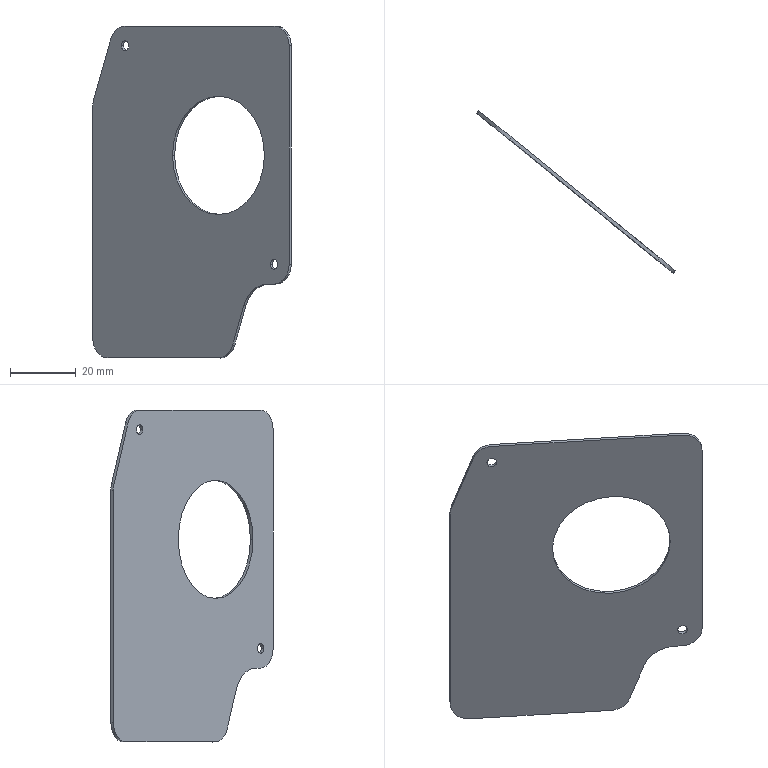Part | SolidWorks | features BaseBody 1 | 1 solid | 34 faces | box 60.39 x 49.373 x 101 mm | volume 6188 mm3 | cylinder 19 | plane 15 | commonest cylinder face diameters 12 x6 3 x4 4.165 x3 3.322 x2 36 x2 0.2 x1
STEP:
#1=CARTESIAN_POINT('',(558.171,-149.274,299.195));
#2=VERTEX_POINT('',#1);
#3=CARTESIAN_POINT('',(530.24,-126.56,299.195));
#4=VERTEX_POINT('',#3);
#5=CARTESIAN_POINT('',(544.205,-137.917,299.195));
#6=DIRECTION('',(0.6309,0.7758,-0.000000012));
#7=DIRECTION('',(-0.7758,0.6309,0.));
#8=AXIS2_PLACEMENT_3D('',#5,#6,#7);
#9=CIRCLE('',#8,18.);
#10=EDGE_CURVE('',#2,#4,#9,.T.);
#11=ORIENTED_EDGE('',*,*,#10,.F.);
#12=CARTESIAN_POINT('',(558.801,-148.498,299.195));
#13=VERTEX_POINT('',#12);
#14=CARTESIAN_POINT('',(558.801,-148.498,299.195));
#15=DIRECTION('',(0.6309,0.7758,-0.000000012));
#16=VECTOR('',#15,1000.);
#17=LINE('',#14,#16);
#18=EDGE_CURVE('',#2,#13,#17,.T.);
#19=ORIENTED_EDGE('',*,*,#18,.T.);
#20=CARTESIAN_POINT('',(530.871,-125.785,299.195));
#21=VERTEX_POINT('',#20);
#22=CARTESIAN_POINT('',(544.836,-137.141,299.195));
#23=DIRECTION('',(-0.6309,-0.7758,0.000000012));
#24=DIRECTION('',(-0.7758,0.6309,0.));
#25=AXIS2_PLACEMENT_3D('',#22,#23,#24);
#26=CIRCLE('',#25,18.);
#27=EDGE_CURVE('',#21,#13,#26,.T.);
#28=ORIENTED_EDGE('',*,*,#27,.F.);
#29=CARTESIAN_POINT('',(530.871,-125.785,299.195));
#30=DIRECTION('',(0.6309,0.7758,-0.000000012));
#31=VECTOR('',#30,1000.);
#32=LINE('',#29,#31);
#33=EDGE_CURVE('',#4,#21,#32,.T.);
#34=ORIENTED_EDGE('',*,*,#33,.F.);
#35=EDGE_LOOP('',(#11,#19,#28,#34));
#36=FACE_OUTER_BOUND('',#35,.T.);
#37=CARTESIAN_POINT('',(544.836,-137.141,299.195));
#38=DIRECTION('',(0.6309,0.7758,-0.000000012));
#39=DIRECTION('',(-0.7758,0.6309,0.));
#40=AXIS2_PLACEMENT_3D('',#37,#38,#39);
#41=CYLINDRICAL_SURFACE('',#40,18.);
#42=ADVANCED_FACE('',(#36),#41,.F.);
#43=CARTESIAN_POINT('',(516.982,-115.778,332.544));
#44=VERTEX_POINT('',#43);
#45=CARTESIAN_POINT('',(514.654,-113.885,332.544));
#46=VERTEX_POINT('',#45);
#47=CARTESIAN_POINT('',(515.818,-114.832,332.544));
#48=DIRECTION('',(0.6309,0.7758,-0.000000012));
#49=DIRECTION('',(-0.7758,0.6309,0.));
#50=AXIS2_PLACEMENT_3D('',#47,#48,#49);
#51=CIRCLE('',#50,1.5);
#52=EDGE_CURVE('',#44,#46,#51,.T.);
#53=ORIENTED_EDGE('',*,*,#52,.F.);
#54=CARTESIAN_POINT('',(517.612,-115.002,332.544));
#55=VERTEX_POINT('',#54);
#56=CARTESIAN_POINT('',(516.982,-115.778,332.544));
#57=DIRECTION('',(0.6309,0.7758,-0.000000012));
#58=VECTOR('',#57,1000.);
#59=LINE('',#56,#58);
#60=EDGE_CURVE('',#44,#55,#59,.T.);
#61=ORIENTED_EDGE('',*,*,#60,.T.);
#62=CARTESIAN_POINT('',(515.285,-113.109,332.544));
#63=VERTEX_POINT('',#62);
#64=CARTESIAN_POINT('',(516.449,-114.056,332.544));
#65=DIRECTION('',(-0.6309,-0.7758,0.000000012));
#66=DIRECTION('',(-0.7758,0.6309,0.));
#67=AXIS2_PLACEMENT_3D('',#64,#65,#66);
#68=CIRCLE('',#67,1.5);
#69=EDGE_CURVE('',#63,#55,#68,.T.);
#70=ORIENTED_EDGE('',*,*,#69,.F.);
#71=CARTESIAN_POINT('',(514.654,-113.885,332.544));
#72=DIRECTION('',(0.6309,0.7758,-0.000000012));
#73=VECTOR('',#72,1000.);
#74=LINE('',#71,#73);
#75=EDGE_CURVE('',#46,#63,#74,.T.);
#76=ORIENTED_EDGE('',*,*,#75,.F.);
#77=EDGE_LOOP('',(#53,#61,#70,#76));
#78=FACE_OUTER_BOUND('',#77,.T.);
#79=CARTESIAN_POINT('',(515.818,-114.832,332.544));
#80=DIRECTION('',(0.6309,0.7758,-0.000000012));
#81=DIRECTION('',(-0.7758,0.6309,0.));
#82=AXIS2_PLACEMENT_3D('',#79,#80,#81);
#83=CYLINDRICAL_SURFACE('',#82,1.5);
#84=ADVANCED_FACE('',(#78),#83,.F.);
#85=CARTESIAN_POINT('',(562.232,-152.577,266.045));
#86=VERTEX_POINT('',#85);
#87=CARTESIAN_POINT('',(559.904,-150.684,266.045));
#88=VERTEX_POINT('',#87);
#89=CARTESIAN_POINT('',(561.068,-151.63,266.045));
#90=DIRECTION('',(0.6309,0.7758,-0.000000012));
#91=DIRECTION('',(-0.7758,0.6309,0.));
#92=AXIS2_PLACEMENT_3D('',#89,#90,#91);
#93=CIRCLE('',#92,1.5);
#94=EDGE_CURVE('',#86,#88,#93,.T.);
#95=ORIENTED_EDGE('',*,*,#94,.F.);
#96=CARTESIAN_POINT('',(562.863,-151.801,266.045));
#97=VERTEX_POINT('',#96);
#98=CARTESIAN_POINT('',(562.358,-152.421,266.045));
#99=DIRECTION('',(0.6309,0.7758,-0.000000012));
#100=VECTOR('',#99,1000.);
#101=LINE('',#98,#100);
#102=EDGE_CURVE('',#86,#97,#101,.T.);
#103=ORIENTED_EDGE('',*,*,#102,.T.);
#104=CARTESIAN_POINT('',(560.535,-149.908,266.045));
#105=VERTEX_POINT('',#104);
#106=CARTESIAN_POINT('',(561.699,-150.854,266.045));
#107=DIRECTION('',(-0.6309,-0.7758,0.000000012));
#108=DIRECTION('',(-0.7758,0.6309,0.));
#109=AXIS2_PLACEMENT_3D('',#106,#107,#108);
#110=CIRCLE('',#109,1.5);
#111=EDGE_CURVE('',#105,#97,#110,.T.);
#112=ORIENTED_EDGE('',*,*,#111,.F.);
#113=CARTESIAN_POINT('',(560.03,-150.529,266.045));
#114=DIRECTION('',(0.6309,0.7758,-0.000000012));
#115=VECTOR('',#114,1000.);
#116=LINE('',#113,#115);
#117=EDGE_CURVE('',#88,#105,#116,.T.);
#118=ORIENTED_EDGE('',*,*,#117,.F.);
#119=EDGE_LOOP('',(#95,#103,#112,#118));
#120=FACE_OUTER_BOUND('',#119,.T.);
#121=CARTESIAN_POINT('',(561.194,-151.475,266.045));
#122=DIRECTION('',(0.6309,0.7758,-0.000000012));
#123=DIRECTION('',(-0.7758,0.6309,0.));
#124=AXIS2_PLACEMENT_3D('',#121,#122,#123);
#125=CYLINDRICAL_SURFACE('',#124,1.5);
#126=ADVANCED_FACE('',(#120),#125,.F.);
#127=CARTESIAN_POINT('',(556.7,-146.789,316.55));
#128=VERTEX_POINT('',#127);
#129=CARTESIAN_POINT('',(556.266,-146.436,317.971));
#130=VERTEX_POINT('',#129);
#131=CARTESIAN_POINT('',(557.881,-147.75,317.971));
#132=DIRECTION('',(0.6309,0.7758,-0.000000012));
#133=DIRECTION('',(0.7758,-0.6309,0.));
#134=AXIS2_PLACEMENT_3D('',#131,#132,#133);
#135=CIRCLE('',#134,2.083);
#136=EDGE_CURVE('',#128,#130,#135,.T.);
#137=ORIENTED_EDGE('',*,*,#136,.T.);
#138=CARTESIAN_POINT('',(556.234,-146.475,317.971));
#139=VERTEX_POINT('',#138);
#140=CARTESIAN_POINT('',(556.266,-146.436,317.971));
#141=DIRECTION('',(-0.6309,-0.7758,0.000000012));
#142=VECTOR('',#141,1000.);
#143=LINE('',#140,#142);
#144=EDGE_CURVE('',#130,#139,#143,.T.);
#145=ORIENTED_EDGE('',*,*,#144,.T.);
#146=CARTESIAN_POINT('',(556.669,-146.828,316.55));
#147=VERTEX_POINT('',#146);
#148=CARTESIAN_POINT('',(557.85,-147.789,317.971));
#149=DIRECTION('',(0.6309,0.7758,-0.000000012));
#150=DIRECTION('',(0.7758,-0.6309,0.));
#151=AXIS2_PLACEMENT_3D('',#148,#149,#150);
#152=CIRCLE('',#151,2.083);
#153=EDGE_CURVE('',#147,#139,#152,.T.);
#154=ORIENTED_EDGE('',*,*,#153,.F.);
#155=CARTESIAN_POINT('',(556.7,-146.789,316.55));
#156=DIRECTION('',(-0.6309,-0.7758,0.000000012));
#157=VECTOR('',#156,1000.);
#158=LINE('',#155,#157);
#159=EDGE_CURVE('',#128,#147,#158,.T.);
#160=ORIENTED_EDGE('',*,*,#159,.F.);
#161=EDGE_LOOP('',(#137,#145,#154,#160));
#162=FACE_OUTER_BOUND('',#161,.T.);
#163=CARTESIAN_POINT('',(557.881,-147.75,317.971));
#164=DIRECTION('',(-0.6309,-0.7758,0.000000012));
#165=DIRECTION('',(0.7758,-0.6309,0.));
#166=AXIS2_PLACEMENT_3D('',#163,#164,#165);
#167=CYLINDRICAL_SURFACE('',#166,2.083);
#168=ADVANCED_FACE('',(#162),#167,.F.);
#169=ORIENTED_EDGE('',*,*,#144,.F.);
#170=CARTESIAN_POINT('',(559.497,-149.064,317.971));
#171=VERTEX_POINT('',#170);
#172=CARTESIAN_POINT('',(557.881,-147.75,317.971));
#173=DIRECTION('',(0.6309,0.7758,-0.000000012));
#174=DIRECTION('',(0.7758,-0.6309,0.));
#175=AXIS2_PLACEMENT_3D('',#172,#173,#174);
#176=CIRCLE('',#175,2.083);
#177=EDGE_CURVE('',#130,#171,#176,.T.);
#178=ORIENTED_EDGE('',*,*,#177,.T.);
#179=CARTESIAN_POINT('',(559.466,-149.103,317.971));
#180=VERTEX_POINT('',#179);
#181=CARTESIAN_POINT('',(559.497,-149.064,317.971));
#182=DIRECTION('',(-0.6309,-0.7758,0.000000012));
#183=VECTOR('',#182,1000.);
#184=LINE('',#181,#183);
#185=EDGE_CURVE('',#171,#180,#184,.T.);
#186=ORIENTED_EDGE('',*,*,#185,.T.);
#187=CARTESIAN_POINT('',(557.85,-147.789,317.971));
#188=DIRECTION('',(0.6309,0.7758,-0.000000012));
#189=DIRECTION('',(0.7758,-0.6309,0.));
#190=AXIS2_PLACEMENT_3D('',#187,#188,#189);
#191=CIRCLE('',#190,2.083);
#192=EDGE_CURVE('',#139,#180,#191,.T.);
#193=ORIENTED_EDGE('',*,*,#192,.F.);
#194=EDGE_LOOP('',(#169,#178,#186,#193));
#195=FACE_OUTER_BOUND('',#194,.T.);
#196=CARTESIAN_POINT('',(557.881,-147.75,317.971));
#197=DIRECTION('',(-0.6309,-0.7758,0.000000012));
#198=DIRECTION('',(0.7758,-0.6309,0.));
#199=AXIS2_PLACEMENT_3D('',#196,#197,#198);
#200=CYLINDRICAL_SURFACE('',#199,2.083);
#201=ADVANCED_FACE('',(#195),#200,.F.);
#202=CARTESIAN_POINT('',(556.561,-146.741,317.971));
#203=VERTEX_POINT('',#202);
#204=CARTESIAN_POINT('',(559.139,-148.837,317.971));
#205=VERTEX_POINT('',#204);
#206=CARTESIAN_POINT('',(557.85,-147.789,317.971));
#207=DIRECTION('',(0.6309,0.7758,-0.000000012));
#208=DIRECTION('',(-0.7758,0.6309,0.));
#209=AXIS2_PLACEMENT_3D('',#206,#207,#208);
#210=CIRCLE('',#209,1.661);
#211=EDGE_CURVE('',#203,#205,#210,.T.);
#212=ORIENTED_EDGE('',*,*,#211,.T.);
#213=CARTESIAN_POINT('',(559.17,-148.798,317.971));
#214=VERTEX_POINT('',#213);
#215=CARTESIAN_POINT('',(559.17,-148.798,317.971));
#216=DIRECTION('',(0.6309,0.7758,-0.000000012));
#217=VECTOR('',#216,1000.);
#218=LINE('',#215,#217);
#219=EDGE_CURVE('',#205,#214,#218,.T.);
#220=ORIENTED_EDGE('',*,*,#219,.T.);
#221=CARTESIAN_POINT('',(556.593,-146.702,317.971));
#222=VERTEX_POINT('',#221);
#223=CARTESIAN_POINT('',(557.881,-147.75,317.971));
#224=DIRECTION('',(-0.6309,-0.7758,0.000000012));
#225=DIRECTION('',(-0.7758,0.6309,0.));
#226=AXIS2_PLACEMENT_3D('',#223,#224,#225);
#227=CIRCLE('',#226,1.661);
#228=EDGE_CURVE('',#214,#222,#227,.T.);
#229=ORIENTED_EDGE('',*,*,#228,.T.);
#230=CARTESIAN_POINT('',(556.593,-146.702,317.971));
#231=DIRECTION('',(0.6309,0.7758,-0.000000012));
#232=VECTOR('',#231,1000.);
#233=LINE('',#230,#232);
#234=EDGE_CURVE('',#203,#222,#233,.T.);
#235=ORIENTED_EDGE('',*,*,#234,.F.);
#236=EDGE_LOOP('',(#212,#220,#229,#235));
#237=FACE_OUTER_BOUND('',#236,.T.);
#238=CARTESIAN_POINT('',(557.881,-147.75,317.971));
#239=DIRECTION('',(0.6309,0.7758,-0.000000012));
#240=DIRECTION('',(-0.7758,0.6309,0.));
#241=AXIS2_PLACEMENT_3D('',#238,#239,#240);
#242=CYLINDRICAL_SURFACE('',#241,1.661);
#243=ADVANCED_FACE('',(#237),#242,.T.);
#244=CARTESIAN_POINT('',(559.205,-150.115,260.045));
#245=VERTEX_POINT('',#244);
#246=CARTESIAN_POINT('',(561.068,-151.63,260.045));
#247=VERTEX_POINT('',#246);
#248=CARTESIAN_POINT('',(535.327,-130.697,260.045));
#249=DIRECTION('',(0.7758,-0.6309,0.));
#250=VECTOR('',#249,1000.);
#251=LINE('',#248,#250);
#252=EDGE_CURVE('',#245,#247,#251,.T.);
#253=ORIENTED_EDGE('',*,*,#252,.T.);
#254=CARTESIAN_POINT('',(565.723,-155.416,266.045));
#255=VERTEX_POINT('',#254);
#256=CARTESIAN_POINT('',(561.068,-151.63,266.045));
#257=DIRECTION('',(-0.6309,-0.7758,0.000000012));
#258=DIRECTION('',(-0.7758,0.6309,0.));
#259=AXIS2_PLACEMENT_3D('',#256,#257,#258);
#260=CIRCLE('',#259,6.);
#261=EDGE_CURVE('',#247,#255,#260,.T.);
#262=ORIENTED_EDGE('',*,*,#261,.T.);
#263=CARTESIAN_POINT('',(565.723,-155.416,332.544));
#264=VERTEX_POINT('',#263);
#265=CARTESIAN_POINT('',(565.723,-155.416,289.016));
#266=DIRECTION('',(0.000000008,0.000000009,1.));
#267=VECTOR('',#266,1000.);
#268=LINE('',#265,#267);
#269=EDGE_CURVE('',#255,#264,#268,.T.);
#270=ORIENTED_EDGE('',*,*,#269,.T.);
#271=CARTESIAN_POINT('',(561.068,-151.63,338.544));
#272=VERTEX_POINT('',#271);
#273=CARTESIAN_POINT('',(561.068,-151.63,332.544));
#274=DIRECTION('',(-0.6309,-0.7758,0.000000012));
#275=DIRECTION('',(-0.7758,0.6309,0.));
#276=AXIS2_PLACEMENT_3D('',#273,#274,#275);
#277=CIRCLE('',#276,6.);
#278=EDGE_CURVE('',#264,#272,#277,.T.);
#279=ORIENTED_EDGE('',*,*,#278,.T.);
#280=CARTESIAN_POINT('',(515.818,-114.832,338.544));
#281=VERTEX_POINT('',#280);
#282=CARTESIAN_POINT('',(535.327,-130.697,338.544));
#283=DIRECTION('',(-0.7758,0.6309,0.));
#284=VECTOR('',#283,1000.);
#285=LINE('',#282,#284);
#286=EDGE_CURVE('',#272,#281,#285,.T.);
#287=ORIENTED_EDGE('',*,*,#286,.T.);
#288=CARTESIAN_POINT('',(511.443,-111.274,334.596));
#289=VERTEX_POINT('',#288);
#290=CARTESIAN_POINT('',(515.818,-114.832,332.544));
#291=DIRECTION('',(-0.6309,-0.7758,0.000000012));
#292=DIRECTION('',(-0.7758,0.6309,0.));
#293=AXIS2_PLACEMENT_3D('',#290,#291,#292);
#294=CIRCLE('',#293,6.);
#295=EDGE_CURVE('',#281,#289,#294,.T.);
#296=ORIENTED_EDGE('',*,*,#295,.T.);
#297=CARTESIAN_POINT('',(506.245,-107.047,316.186));
#298=VERTEX_POINT('',#297);
#299=CARTESIAN_POINT('',(511.443,-111.274,334.596));
#300=DIRECTION('',(-0.2654,0.2158,-0.9397));
#301=VECTOR('',#300,1000.);
#302=LINE('',#299,#301);
#303=EDGE_CURVE('',#289,#298,#302,.T.);
#304=ORIENTED_EDGE('',*,*,#303,.T.);
#305=CARTESIAN_POINT('',(505.964,-106.818,314.134));
#306=VERTEX_POINT('',#305);
#307=CARTESIAN_POINT('',(510.619,-110.604,314.134));
#308=DIRECTION('',(-0.6309,-0.7758,0.000000012));
#309=DIRECTION('',(-0.7758,0.6309,0.));
#310=AXIS2_PLACEMENT_3D('',#307,#308,#309);
#311=CIRCLE('',#310,6.);
#312=EDGE_CURVE('',#298,#306,#311,.T.);
#313=ORIENTED_EDGE('',*,*,#312,.T.);
#314=CARTESIAN_POINT('',(505.964,-106.818,243.545));
#315=VERTEX_POINT('',#314);
#316=CARTESIAN_POINT('',(505.964,-106.818,289.016));
#317=DIRECTION('',(-0.000000008,-0.000000009,-1.));
#318=VECTOR('',#317,1000.);
#319=LINE('',#316,#318);
#320=EDGE_CURVE('',#306,#315,#319,.T.);
#321=ORIENTED_EDGE('',*,*,#320,.T.);
#322=CARTESIAN_POINT('',(510.619,-110.604,237.545));
#323=VERTEX_POINT('',#322);
#324=CARTESIAN_POINT('',(510.619,-110.604,243.545));
#325=DIRECTION('',(-0.6309,-0.7758,0.000000012));
#326=DIRECTION('',(-0.7758,0.6309,0.));
#327=AXIS2_PLACEMENT_3D('',#324,#325,#326);
#328=CIRCLE('',#327,6.);
#329=EDGE_CURVE('',#315,#323,#328,.T.);
#330=ORIENTED_EDGE('',*,*,#329,.T.);
#331=CARTESIAN_POINT('',(544.159,-137.879,237.545));
#332=VERTEX_POINT('',#331);
#333=CARTESIAN_POINT('',(535.327,-130.697,237.545));
#334=DIRECTION('',(0.7758,-0.6309,0.));
#335=VECTOR('',#334,1000.);
#336=LINE('',#333,#335);
#337=EDGE_CURVE('',#323,#332,#336,.T.);
#338=ORIENTED_EDGE('',*,*,#337,.T.);
#339=CARTESIAN_POINT('',(548.533,-141.437,241.492));
#340=VERTEX_POINT('',#339);
#341=CARTESIAN_POINT('',(544.159,-137.879,243.545));
#342=DIRECTION('',(-0.6309,-0.7758,0.000000012));
#343=DIRECTION('',(-0.7758,0.6309,0.));
#344=AXIS2_PLACEMENT_3D('',#341,#342,#343);
#345=CIRCLE('',#344,6.);
#346=EDGE_CURVE('',#332,#340,#345,.T.);
#347=ORIENTED_EDGE('',*,*,#346,.T.);
#348=CARTESIAN_POINT('',(551.914,-144.186,253.465));
#349=VERTEX_POINT('',#348);
#350=CARTESIAN_POINT('',(548.533,-141.437,241.492));
#351=DIRECTION('',(0.2654,-0.2158,0.9397));
#352=VECTOR('',#351,1000.);
#353=LINE('',#350,#352);
#354=EDGE_CURVE('',#340,#349,#353,.T.);
#355=ORIENTED_EDGE('',*,*,#354,.T.);
#356=CARTESIAN_POINT('',(559.205,-150.115,250.045));
#357=DIRECTION('',(0.6309,0.7758,-0.000000012));
#358=DIRECTION('',(0.7758,-0.6309,0.));
#359=AXIS2_PLACEMENT_3D('',#356,#357,#358);
#360=CIRCLE('',#359,10.);
#361=EDGE_CURVE('',#349,#245,#360,.T.);
#362=ORIENTED_EDGE('',*,*,#361,.T.);
#363=EDGE_LOOP('',(#253,#262,#270,#279,#287,#296,#304,#313,#321,#330,#338,#347,#355,#362));
#364=FACE_OUTER_BOUND('',#363,.T.);
#365=CARTESIAN_POINT('',(544.205,-137.917,299.195));
#366=DIRECTION('',(0.6309,0.7758,-0.000000012));
#367=DIRECTION('',(-0.7758,0.6309,0.));
#368=AXIS2_PLACEMENT_3D('',#365,#366,#367);
#369=CIRCLE('',#368,18.);
#370=EDGE_CURVE('',#4,#2,#369,.T.);
#371=ORIENTED_EDGE('',*,*,#370,.T.);
#372=ORIENTED_EDGE('',*,*,#10,.T.);
#373=EDGE_LOOP('',(#371,#372));
#374=FACE_BOUND('',#373,.T.);
#375=CARTESIAN_POINT('',(515.818,-114.832,332.544));
#376=DIRECTION('',(0.6309,0.7758,-0.000000012));
#377=DIRECTION('',(-0.7758,0.6309,0.));
#378=AXIS2_PLACEMENT_3D('',#375,#376,#377);
#379=CIRCLE('',#378,1.5);
#380=EDGE_CURVE('',#46,#44,#379,.T.);
#381=ORIENTED_EDGE('',*,*,#380,.T.);
#382=ORIENTED_EDGE('',*,*,#52,.T.);
#383=EDGE_LOOP('',(#381,#382));
#384=FACE_BOUND('',#383,.T.);
#385=CARTESIAN_POINT('',(561.068,-151.63,266.045));
#386=DIRECTION('',(0.6309,0.7758,-0.000000012));
#387=DIRECTION('',(-0.7758,0.6309,0.));
#388=AXIS2_PLACEMENT_3D('',#385,#386,#387);
#389=CIRCLE('',#388,1.5);
#390=EDGE_CURVE('',#88,#86,#389,.T.);
#391=ORIENTED_EDGE('',*,*,#390,.T.);
#392=ORIENTED_EDGE('',*,*,#94,.T.);
#393=EDGE_LOOP('',(#391,#392));
#394=FACE_BOUND('',#393,.T.);
#395=CARTESIAN_POINT('',(535.327,-130.697,289.016));
#396=DIRECTION('',(-0.6309,-0.7758,0.000000012));
#397=DIRECTION('',(0.7758,-0.6309,0.));
#398=AXIS2_PLACEMENT_3D('',#395,#396,#397);
#399=PLANE('',#398);
#400=ADVANCED_FACE('',(#364,#374,#384,#394),#399,.T.);
#401=CARTESIAN_POINT('',(561.699,-150.854,260.045));
#402=VERTEX_POINT('',#401);
#403=CARTESIAN_POINT('',(561.068,-151.63,260.045));
#404=DIRECTION('',(0.6309,0.7758,-0.000000012));
#405=VECTOR('',#404,1000.);
#406=LINE('',#403,#405);
#407=EDGE_CURVE('',#247,#402,#406,.T.);
#408=ORIENTED_EDGE('',*,*,#407,.T.);
#409=CARTESIAN_POINT('',(566.354,-154.64,266.045));
#410=VERTEX_POINT('',#409);
#411=CARTESIAN_POINT('',(561.699,-150.854,266.045));
#412=DIRECTION('',(-0.6309,-0.7758,0.000000012));
#413=DIRECTION('',(-0.7758,0.6309,0.));
#414=AXIS2_PLACEMENT_3D('',#411,#412,#413);
#415=CIRCLE('',#414,6.);
#416=EDGE_CURVE('',#402,#410,#415,.T.);
#417=ORIENTED_EDGE('',*,*,#416,.T.);
#418=CARTESIAN_POINT('',(565.723,-155.416,266.045));
#419=DIRECTION('',(-0.6309,-0.7758,0.));
#420=VECTOR('',#419,1000.);
#421=LINE('',#418,#420);
#422=EDGE_CURVE('',#410,#255,#421,.T.);
#423=ORIENTED_EDGE('',*,*,#422,.T.);
#424=ORIENTED_EDGE('',*,*,#261,.F.);
#425=EDGE_LOOP('',(#408,#417,#423,#424));
#426=FACE_OUTER_BOUND('',#425,.T.);
#427=CARTESIAN_POINT('',(561.068,-151.63,266.045));
#428=DIRECTION('',(0.6309,0.7758,-0.000000012));
#429=DIRECTION('',(-0.7758,0.6309,0.));
#430=AXIS2_PLACEMENT_3D('',#427,#428,#429);
#431=CYLINDRICAL_SURFACE('',#430,6.);
#432=ADVANCED_FACE('',(#426),#431,.T.);
#433=CARTESIAN_POINT('',(559.835,-149.339,260.045));
#434=VERTEX_POINT('',#433);
#435=CARTESIAN_POINT('',(559.835,-149.339,260.045));
#436=DIRECTION('',(-0.6309,-0.7758,0.000000012));
#437=VECTOR('',#436,1000.);
#438=LINE('',#435,#437);
#439=EDGE_CURVE('',#434,#245,#438,.T.);
#440=ORIENTED_EDGE('',*,*,#439,.F.);
#441=CARTESIAN_POINT('',(561.699,-150.854,260.045));
#442=DIRECTION('',(-0.7758,0.6309,0.000000021));
#443=VECTOR('',#442,1000.);
#444=LINE('',#441,#443);
#445=EDGE_CURVE('',#402,#434,#444,.T.);
#446=ORIENTED_EDGE('',*,*,#445,.F.);
#447=ORIENTED_EDGE('',*,*,#407,.F.);
#448=ORIENTED_EDGE('',*,*,#252,.F.);
#449=EDGE_LOOP('',(#440,#446,#447,#448));
#450=FACE_OUTER_BOUND('',#449,.T.);
#451=CARTESIAN_POINT('',(560.136,-150.873,260.045));
#452=DIRECTION('',(0.000000024,-0.000000004,1.));
#453=DIRECTION('',(1.,0.,-0.000000024));
#454=AXIS2_PLACEMENT_3D('',#451,#452,#453);
#455=PLANE('',#454);
#456=ADVANCED_FACE('',(#450),#455,.F.);
#457=CARTESIAN_POINT('',(552.545,-143.41,253.465));
#458=VERTEX_POINT('',#457);
#459=CARTESIAN_POINT('',(559.835,-149.339,250.045));
#460=DIRECTION('',(-0.6309,-0.7758,0.000000012));
#461=DIRECTION('',(0.7758,-0.6309,0.));
#462=AXIS2_PLACEMENT_3D('',#459,#460,#461);
#463=CIRCLE('',#462,10.);
#464=EDGE_CURVE('',#434,#458,#463,.T.);
#465=ORIENTED_EDGE('',*,*,#464,.F.);
#466=ORIENTED_EDGE('',*,*,#439,.T.);
#467=ORIENTED_EDGE('',*,*,#361,.F.);
#468=CARTESIAN_POINT('',(551.914,-144.186,253.465));
#469=DIRECTION('',(-0.6309,-0.7758,0.000000012));
#470=VECTOR('',#469,1000.);
#471=LINE('',#468,#470);
#472=EDGE_CURVE('',#458,#349,#471,.T.);
#473=ORIENTED_EDGE('',*,*,#472,.F.);
#474=EDGE_LOOP('',(#465,#466,#467,#473));
#475=FACE_OUTER_BOUND('',#474,.T.);
#476=CARTESIAN_POINT('',(559.205,-150.115,250.045));
#477=DIRECTION('',(-0.6309,-0.7758,0.000000012));
#478=DIRECTION('',(0.7758,-0.6309,0.));
#479=AXIS2_PLACEMENT_3D('',#476,#477,#478);
#480=CYLINDRICAL_SURFACE('',#479,10.);
#481=ADVANCED_FACE('',(#475),#480,.F.);
#482=CARTESIAN_POINT('',(549.164,-140.661,241.492));
#483=VERTEX_POINT('',#482);
#484=CARTESIAN_POINT('',(548.533,-141.437,241.492));
#485=DIRECTION('',(-0.6309,-0.7758,0.));
#486=VECTOR('',#485,1000.);
#487=LINE('',#484,#486);
#488=EDGE_CURVE('',#483,#340,#487,.T.);
#489=ORIENTED_EDGE('',*,*,#488,.F.);
#490=CARTESIAN_POINT('',(550.855,-142.036,247.479));
#491=DIRECTION('',(-0.2654,0.2158,-0.9397));
#492=VECTOR('',#491,1000.);
#493=LINE('',#490,#492);
#494=EDGE_CURVE('',#458,#483,#493,.T.);
#495=ORIENTED_EDGE('',*,*,#494,.F.);
#496=ORIENTED_EDGE('',*,*,#472,.T.);
#497=ORIENTED_EDGE('',*,*,#354,.F.);
#498=EDGE_LOOP('',(#489,#495,#496,#497));
#499=FACE_OUTER_BOUND('',#498,.T.);
#500=CARTESIAN_POINT('',(550.224,-142.811,247.479));
#501=DIRECTION('',(-0.7291,0.5929,0.342));
#502=DIRECTION('',(-0.6309,-0.7758,0.));
#503=AXIS2_PLACEMENT_3D('',#500,#501,#502);
#504=PLANE('',#503);
#505=ADVANCED_FACE('',(#499),#504,.F.);
#506=ORIENTED_EDGE('',*,*,#488,.T.);
#507=ORIENTED_EDGE('',*,*,#346,.F.);
#508=CARTESIAN_POINT('',(544.79,-137.104,237.545));
#509=VERTEX_POINT('',#508);
#510=CARTESIAN_POINT('',(544.159,-137.879,237.545));
#511=DIRECTION('',(0.6309,0.7758,-0.000000012));
#512=VECTOR('',#511,1000.);
#513=LINE('',#510,#512);
#514=EDGE_CURVE('',#332,#509,#513,.T.);
#515=ORIENTED_EDGE('',*,*,#514,.T.);
#516=CARTESIAN_POINT('',(544.79,-137.104,243.545));
#517=DIRECTION('',(-0.6309,-0.7758,0.000000012));
#518=DIRECTION('',(-0.7758,0.6309,0.));
#519=AXIS2_PLACEMENT_3D('',#516,#517,#518);
#520=CIRCLE('',#519,6.);
#521=EDGE_CURVE('',#509,#483,#520,.T.);
#522=ORIENTED_EDGE('',*,*,#521,.T.);
#523=EDGE_LOOP('',(#506,#507,#515,#522));
#524=FACE_OUTER_BOUND('',#523,.T.);
#525=CARTESIAN_POINT('',(544.159,-137.879,243.545));
#526=DIRECTION('',(0.6309,0.7758,-0.000000012));
#527=DIRECTION('',(-0.7758,0.6309,0.));
#528=AXIS2_PLACEMENT_3D('',#525,#526,#527);
#529=CYLINDRICAL_SURFACE('',#528,6.);
#530=ADVANCED_FACE('',(#524),#529,.T.);
#531=CARTESIAN_POINT('',(511.25,-109.828,237.545));
#532=VERTEX_POINT('',#531);
#533=CARTESIAN_POINT('',(511.25,-109.828,237.545));
#534=DIRECTION('',(-0.6309,-0.7758,0.000000012));
#535=VECTOR('',#534,1000.);
#536=LINE('',#533,#535);
#537=EDGE_CURVE('',#532,#323,#536,.T.);
#538=ORIENTED_EDGE('',*,*,#537,.F.);
#539=CARTESIAN_POINT('',(544.79,-137.104,237.545));
#540=DIRECTION('',(-0.7758,0.6309,0.000000021));
#541=VECTOR('',#540,1000.);
#542=LINE('',#539,#541);
#543=EDGE_CURVE('',#509,#532,#542,.T.);
#544=ORIENTED_EDGE('',*,*,#543,.F.);
#545=ORIENTED_EDGE('',*,*,#514,.F.);
#546=ORIENTED_EDGE('',*,*,#337,.F.);
#547=EDGE_LOOP('',(#538,#544,#545,#546));
#548=FACE_OUTER_BOUND('',#547,.T.);
#549=CARTESIAN_POINT('',(527.389,-124.242,237.545));
#550=DIRECTION('',(0.000000024,-0.000000004,1.));
#551=DIRECTION('',(1.,0.,-0.000000024));
#552=AXIS2_PLACEMENT_3D('',#549,#550,#551);
#553=PLANE('',#552);
#554=ADVANCED_FACE('',(#548),#553,.F.);
#555=ORIENTED_EDGE('',*,*,#537,.T.);
#556=ORIENTED_EDGE('',*,*,#329,.F.);
#557=CARTESIAN_POINT('',(506.595,-106.043,243.545));
#558=VERTEX_POINT('',#557);
#559=CARTESIAN_POINT('',(505.964,-106.818,243.545));
#560=DIRECTION('',(0.6309,0.7758,-0.000000012));
#561=VECTOR('',#560,1000.);
#562=LINE('',#559,#561);
#563=EDGE_CURVE('',#315,#558,#562,.T.);
#564=ORIENTED_EDGE('',*,*,#563,.T.);
#565=CARTESIAN_POINT('',(511.25,-109.828,243.545));
#566=DIRECTION('',(-0.6309,-0.7758,0.000000012));
#567=DIRECTION('',(-0.7758,0.6309,0.));
#568=AXIS2_PLACEMENT_3D('',#565,#566,#567);
#569=CIRCLE('',#568,6.);
#570=EDGE_CURVE('',#558,#532,#569,.T.);
#571=ORIENTED_EDGE('',*,*,#570,.T.);
#572=EDGE_LOOP('',(#555,#556,#564,#571));
#573=FACE_OUTER_BOUND('',#572,.T.);
#574=CARTESIAN_POINT('',(510.619,-110.604,243.545));
#575=DIRECTION('',(0.6309,0.7758,-0.000000012));
#576=DIRECTION('',(-0.7758,0.6309,0.));
#577=AXIS2_PLACEMENT_3D('',#574,#575,#576);
#578=CYLINDRICAL_SURFACE('',#577,6.);
#579=ADVANCED_FACE('',(#573),#578,.T.);
#580=CARTESIAN_POINT('',(506.595,-106.043,314.134));
#581=VERTEX_POINT('',#580);
#582=CARTESIAN_POINT('',(505.964,-106.818,314.134));
#583=DIRECTION('',(-0.6309,-0.7758,0.));
#584=VECTOR('',#583,1000.);
#585=LINE('',#582,#584);
#586=EDGE_CURVE('',#581,#306,#585,.T.);
#587=ORIENTED_EDGE('',*,*,#586,.F.);
#588=CARTESIAN_POINT('',(506.595,-106.043,278.839));
#589=DIRECTION('',(0.000000016,-0.000000013,1.));
#590=VECTOR('',#589,1000.);
#591=LINE('',#588,#590);
#592=EDGE_CURVE('',#558,#581,#591,.T.);
#593=ORIENTED_EDGE('',*,*,#592,.F.);
#594=ORIENTED_EDGE('',*,*,#563,.F.);
#595=ORIENTED_EDGE('',*,*,#320,.F.);
#596=EDGE_LOOP('',(#587,#593,#594,#595));
#597=FACE_OUTER_BOUND('',#596,.T.);
#598=CARTESIAN_POINT('',(505.964,-106.818,278.839));
#599=DIRECTION('',(0.7758,-0.6309,-0.000000021));
#600=DIRECTION('',(0.6309,0.7758,0.));
#601=AXIS2_PLACEMENT_3D('',#598,#599,#600);
#602=PLANE('',#601);
#603=ADVANCED_FACE('',(#597),#602,.F.);
#604=ORIENTED_EDGE('',*,*,#586,.T.);
#605=ORIENTED_EDGE('',*,*,#312,.F.);
#606=CARTESIAN_POINT('',(506.876,-106.271,316.186));
#607=VERTEX_POINT('',#606);
#608=CARTESIAN_POINT('',(506.245,-107.047,316.186));
#609=DIRECTION('',(0.6309,0.7758,-0.000000012));
#610=VECTOR('',#609,1000.);
#611=LINE('',#608,#610);
#612=EDGE_CURVE('',#298,#607,#611,.T.);
#613=ORIENTED_EDGE('',*,*,#612,.T.);
#614=CARTESIAN_POINT('',(511.25,-109.828,314.134));
#615=DIRECTION('',(-0.6309,-0.7758,0.000000012));
#616=DIRECTION('',(-0.7758,0.6309,0.));
#617=AXIS2_PLACEMENT_3D('',#614,#615,#616);
#618=CIRCLE('',#617,6.);
#619=EDGE_CURVE('',#607,#581,#618,.T.);
#620=ORIENTED_EDGE('',*,*,#619,.T.);
#621=EDGE_LOOP('',(#604,#605,#613,#620));
#622=FACE_OUTER_BOUND('',#621,.T.);
#623=CARTESIAN_POINT('',(510.619,-110.604,314.134));
#624=DIRECTION('',(0.6309,0.7758,-0.000000012));
#625=DIRECTION('',(-0.7758,0.6309,0.));
#626=AXIS2_PLACEMENT_3D('',#623,#624,#625);
#627=CYLINDRICAL_SURFACE('',#626,6.);
#628=ADVANCED_FACE('',(#622),#627,.T.);
#629=CARTESIAN_POINT('',(512.074,-110.499,334.596));
#630=VERTEX_POINT('',#629);
#631=CARTESIAN_POINT('',(511.443,-111.274,334.596));
#632=DIRECTION('',(-0.6309,-0.7758,0.));
#633=VECTOR('',#632,1000.);
#634=LINE('',#631,#633);
#635=EDGE_CURVE('',#630,#289,#634,.T.);
#636=ORIENTED_EDGE('',*,*,#635,.F.);
#637=CARTESIAN_POINT('',(509.475,-108.385,325.391));
#638=DIRECTION('',(0.2654,-0.2158,0.9397));
#639=VECTOR('',#638,1000.);
#640=LINE('',#637,#639);
#641=EDGE_CURVE('',#607,#630,#640,.T.);
#642=ORIENTED_EDGE('',*,*,#641,.F.);
#643=ORIENTED_EDGE('',*,*,#612,.F.);
#644=ORIENTED_EDGE('',*,*,#303,.F.);
#645=EDGE_LOOP('',(#636,#642,#643,#644));
#646=FACE_OUTER_BOUND('',#645,.T.);
#647=CARTESIAN_POINT('',(508.844,-109.161,325.391));
#648=DIRECTION('',(0.7291,-0.5929,-0.342));
#649=DIRECTION('',(0.6309,0.7758,0.));
#650=AXIS2_PLACEMENT_3D('',#647,#648,#649);
#651=PLANE('',#650);
#652=ADVANCED_FACE('',(#646),#651,.F.);
#653=ORIENTED_EDGE('',*,*,#635,.T.);
#654=ORIENTED_EDGE('',*,*,#295,.F.);
#655=CARTESIAN_POINT('',(516.449,-114.056,338.544));
#656=VERTEX_POINT('',#655);
#657=CARTESIAN_POINT('',(515.818,-114.832,338.544));
#658=DIRECTION('',(0.6309,0.7758,-0.000000012));
#659=VECTOR('',#658,1000.);
#660=LINE('',#657,#659);
#661=EDGE_CURVE('',#281,#656,#660,.T.);
#662=ORIENTED_EDGE('',*,*,#661,.T.);
#663=CARTESIAN_POINT('',(516.449,-114.056,332.544));
#664=DIRECTION('',(-0.6309,-0.7758,0.000000012));
#665=DIRECTION('',(-0.7758,0.6309,0.));
#666=AXIS2_PLACEMENT_3D('',#663,#664,#665);
#667=CIRCLE('',#666,6.);
#668=EDGE_CURVE('',#656,#630,#667,.T.);
#669=ORIENTED_EDGE('',*,*,#668,.T.);
#670=EDGE_LOOP('',(#653,#654,#662,#669));
#671=FACE_OUTER_BOUND('',#670,.T.);
#672=CARTESIAN_POINT('',(515.818,-114.832,332.544));
#673=DIRECTION('',(0.6309,0.7758,-0.000000012));
#674=DIRECTION('',(-0.7758,0.6309,0.));
#675=AXIS2_PLACEMENT_3D('',#672,#673,#674);
#676=CYLINDRICAL_SURFACE('',#675,6.);
#677=ADVANCED_FACE('',(#671),#676,.T.);
#678=CARTESIAN_POINT('',(561.699,-150.854,338.544));
#679=VERTEX_POINT('',#678);
#680=CARTESIAN_POINT('',(561.699,-150.854,338.544));
#681=DIRECTION('',(-0.6309,-0.7758,0.000000012));
#682=VECTOR('',#681,1000.);
#683=LINE('',#680,#682);
#684=EDGE_CURVE('',#679,#272,#683,.T.);
#685=ORIENTED_EDGE('',*,*,#684,.F.);
#686=CARTESIAN_POINT('',(516.449,-114.056,338.544));
#687=DIRECTION('',(0.7758,-0.6309,-0.000000021));
#688=VECTOR('',#687,1000.);
#689=LINE('',#686,#688);
#690=EDGE_CURVE('',#656,#679,#689,.T.);
#691=ORIENTED_EDGE('',*,*,#690,.F.);
#692=ORIENTED_EDGE('',*,*,#661,.F.);
#693=ORIENTED_EDGE('',*,*,#286,.F.);
#694=EDGE_LOOP('',(#685,#691,#692,#693));
#695=FACE_OUTER_BOUND('',#694,.T.);
#696=CARTESIAN_POINT('',(538.443,-133.231,338.544));
#697=DIRECTION('',(-0.000000024,0.000000004,-1.));
#698=DIRECTION('',(-1.,0.,0.000000024));
#699=AXIS2_PLACEMENT_3D('',#696,#697,#698);
#700=PLANE('',#699);
#701=ADVANCED_FACE('',(#695),#700,.F.);
#702=ORIENTED_EDGE('',*,*,#684,.T.);
#703=ORIENTED_EDGE('',*,*,#278,.F.);
#704=CARTESIAN_POINT('',(566.354,-154.64,332.544));
#705=VERTEX_POINT('',#704);
#706=CARTESIAN_POINT('',(565.723,-155.416,332.544));
#707=DIRECTION('',(0.6309,0.7758,-0.000000012));
#708=VECTOR('',#707,1000.);
#709=LINE('',#706,#708);
#710=EDGE_CURVE('',#264,#705,#709,.T.);
#711=ORIENTED_EDGE('',*,*,#710,.T.);
#712=CARTESIAN_POINT('',(561.699,-150.854,332.544));
#713=DIRECTION('',(-0.6309,-0.7758,0.000000012));
#714=DIRECTION('',(-0.7758,0.6309,0.));
#715=AXIS2_PLACEMENT_3D('',#712,#713,#714);
#716=CIRCLE('',#715,6.);
#717=EDGE_CURVE('',#705,#679,#716,.T.);
#718=ORIENTED_EDGE('',*,*,#717,.T.);
#719=EDGE_LOOP('',(#702,#703,#711,#718));
#720=FACE_OUTER_BOUND('',#719,.T.);
#721=CARTESIAN_POINT('',(561.068,-151.63,332.544));
#722=DIRECTION('',(0.6309,0.7758,-0.000000012));
#723=DIRECTION('',(-0.7758,0.6309,0.));
#724=AXIS2_PLACEMENT_3D('',#721,#722,#723);
#725=CYLINDRICAL_SURFACE('',#724,6.);
#726=ADVANCED_FACE('',(#720),#725,.T.);
#727=ORIENTED_EDGE('',*,*,#422,.F.);
#728=CARTESIAN_POINT('',(566.354,-154.64,299.294));
#729=DIRECTION('',(-0.000000016,0.000000013,-1.));
#730=VECTOR('',#729,1000.);
#731=LINE('',#728,#730);
#732=EDGE_CURVE('',#705,#410,#731,.T.);
#733=ORIENTED_EDGE('',*,*,#732,.F.);
#734=ORIENTED_EDGE('',*,*,#710,.F.);
#735=ORIENTED_EDGE('',*,*,#269,.F.);
#736=EDGE_LOOP('',(#727,#733,#734,#735));
#737=FACE_OUTER_BOUND('',#736,.T.);
#738=CARTESIAN_POINT('',(565.723,-155.416,299.294));
#739=DIRECTION('',(-0.7758,0.6309,0.000000021));
#740=DIRECTION('',(-0.6309,-0.7758,0.));
#741=AXIS2_PLACEMENT_3D('',#738,#739,#740);
#742=PLANE('',#741);
#743=ADVANCED_FACE('',(#737),#742,.F.);
#744=ORIENTED_EDGE('',*,*,#18,.F.);
#745=ORIENTED_EDGE('',*,*,#370,.F.);
#746=ORIENTED_EDGE('',*,*,#33,.T.);
#747=CARTESIAN_POINT('',(544.836,-137.141,299.195));
#748=DIRECTION('',(-0.6309,-0.7758,0.000000012));
#749=DIRECTION('',(-0.7758,0.6309,0.));
#750=AXIS2_PLACEMENT_3D('',#747,#748,#749);
#751=CIRCLE('',#750,18.);
#752=EDGE_CURVE('',#13,#21,#751,.T.);
#753=ORIENTED_EDGE('',*,*,#752,.F.);
#754=EDGE_LOOP('',(#744,#745,#746,#753));
#755=FACE_OUTER_BOUND('',#754,.T.);
#756=CARTESIAN_POINT('',(544.836,-137.141,299.195));
#757=DIRECTION('',(0.6309,0.7758,-0.000000012));
#758=DIRECTION('',(-0.7758,0.6309,0.));
#759=AXIS2_PLACEMENT_3D('',#756,#757,#758);
#760=CYLINDRICAL_SURFACE('',#759,18.);
#761=ADVANCED_FACE('',(#755),#760,.F.);
#762=ORIENTED_EDGE('',*,*,#60,.F.);
#763=ORIENTED_EDGE('',*,*,#380,.F.);
#764=ORIENTED_EDGE('',*,*,#75,.T.);
#765=CARTESIAN_POINT('',(516.449,-114.056,332.544));
#766=DIRECTION('',(-0.6309,-0.7758,0.000000012));
#767=DIRECTION('',(-0.7758,0.6309,0.));
#768=AXIS2_PLACEMENT_3D('',#765,#766,#767);
#769=CIRCLE('',#768,1.5);
#770=EDGE_CURVE('',#55,#63,#769,.T.);
#771=ORIENTED_EDGE('',*,*,#770,.F.);
#772=EDGE_LOOP('',(#762,#763,#764,#771));
#773=FACE_OUTER_BOUND('',#772,.T.);
#774=CARTESIAN_POINT('',(515.818,-114.832,332.544));
#775=DIRECTION('',(0.6309,0.7758,-0.000000012));
#776=DIRECTION('',(-0.7758,0.6309,0.));
#777=AXIS2_PLACEMENT_3D('',#774,#775,#776);
#778=CYLINDRICAL_SURFACE('',#777,1.5);
#779=ADVANCED_FACE('',(#773),#778,.F.);
#780=ORIENTED_EDGE('',*,*,#102,.F.);
#781=ORIENTED_EDGE('',*,*,#390,.F.);
#782=ORIENTED_EDGE('',*,*,#117,.T.);
#783=CARTESIAN_POINT('',(561.699,-150.854,266.045));
#784=DIRECTION('',(-0.6309,-0.7758,0.000000012));
#785=DIRECTION('',(-0.7758,0.6309,0.));
#786=AXIS2_PLACEMENT_3D('',#783,#784,#785);
#787=CIRCLE('',#786,1.5);
#788=EDGE_CURVE('',#97,#105,#787,.T.);
#789=ORIENTED_EDGE('',*,*,#788,.F.);
#790=EDGE_LOOP('',(#780,#781,#782,#789));
#791=FACE_OUTER_BOUND('',#790,.T.);
#792=CARTESIAN_POINT('',(561.194,-151.475,266.045));
#793=DIRECTION('',(0.6309,0.7758,-0.000000012));
#794=DIRECTION('',(-0.7758,0.6309,0.));
#795=AXIS2_PLACEMENT_3D('',#792,#793,#794);
#796=CYLINDRICAL_SURFACE('',#795,1.5);
#797=ADVANCED_FACE('',(#791),#796,.F.);
#798=ORIENTED_EDGE('',*,*,#416,.F.);
#799=ORIENTED_EDGE('',*,*,#445,.T.);
#800=ORIENTED_EDGE('',*,*,#464,.T.);
#801=ORIENTED_EDGE('',*,*,#494,.T.);
#802=ORIENTED_EDGE('',*,*,#521,.F.);
#803=ORIENTED_EDGE('',*,*,#543,.T.);
#804=ORIENTED_EDGE('',*,*,#570,.F.);
#805=ORIENTED_EDGE('',*,*,#592,.T.);
#806=ORIENTED_EDGE('',*,*,#619,.F.);
#807=ORIENTED_EDGE('',*,*,#641,.T.);
#808=ORIENTED_EDGE('',*,*,#668,.F.);
#809=ORIENTED_EDGE('',*,*,#690,.T.);
#810=ORIENTED_EDGE('',*,*,#717,.F.);
#811=ORIENTED_EDGE('',*,*,#732,.T.);
#812=EDGE_LOOP('',(#798,#799,#800,#801,#802,#803,#804,#805,#806,#807,#808,#809,#810,#811));
#813=FACE_OUTER_BOUND('',#812,.T.);
#814=ORIENTED_EDGE('',*,*,#27,.T.);
#815=ORIENTED_EDGE('',*,*,#752,.T.);
#816=EDGE_LOOP('',(#814,#815));
#817=FACE_BOUND('',#816,.T.);
#818=ORIENTED_EDGE('',*,*,#69,.T.);
#819=ORIENTED_EDGE('',*,*,#770,.T.);
#820=EDGE_LOOP('',(#818,#819));
#821=FACE_BOUND('',#820,.T.);
#822=ORIENTED_EDGE('',*,*,#111,.T.);
#823=ORIENTED_EDGE('',*,*,#788,.T.);
#824=EDGE_LOOP('',(#822,#823));
#825=FACE_BOUND('',#824,.T.);
#826=ORIENTED_EDGE('',*,*,#136,.F.);
#827=CARTESIAN_POINT('',(555.321,-145.668,314.539));
#828=VERTEX_POINT('',#827);
#829=CARTESIAN_POINT('',(555.321,-145.668,314.539));
#830=DIRECTION('',(0.5138,-0.4178,0.7493));
#831=VECTOR('',#830,1000.);
#832=LINE('',#829,#831);
#833=EDGE_CURVE('',#828,#128,#832,.T.);
#834=ORIENTED_EDGE('',*,*,#833,.F.);
#835=CARTESIAN_POINT('',(555.128,-145.511,314.103));
#836=VERTEX_POINT('',#835);
#837=CARTESIAN_POINT('',(555.128,-145.511,314.103));
#838=DIRECTION('',(0.3849,-0.313,0.8683));
#839=VECTOR('',#838,1000.);
#840=LINE('',#837,#839);
#841=EDGE_CURVE('',#836,#828,#840,.T.);
#842=ORIENTED_EDGE('',*,*,#841,.F.);
#843=CARTESIAN_POINT('',(555.242,-145.603,313.973));
#844=VERTEX_POINT('',#843);
#845=CARTESIAN_POINT('',(555.195,-145.565,314.053));
#846=DIRECTION('',(0.6309,0.7758,-0.000000012));
#847=DIRECTION('',(0.7758,-0.6309,0.));
#848=AXIS2_PLACEMENT_3D('',#845,#846,#847);
#849=CIRCLE('',#848,0.1);
#850=EDGE_CURVE('',#844,#836,#849,.T.);
#851=ORIENTED_EDGE('',*,*,#850,.F.);
#852=CARTESIAN_POINT('',(555.554,-145.857,314.274));
#853=VERTEX_POINT('',#852);
#854=CARTESIAN_POINT('',(555.554,-145.857,314.274));
#855=DIRECTION('',(-0.6212,0.5051,-0.5991));
#856=VECTOR('',#855,1000.);
#857=LINE('',#854,#856);
#858=EDGE_CURVE('',#853,#844,#857,.T.);
#859=ORIENTED_EDGE('',*,*,#858,.F.);
#860=CARTESIAN_POINT('',(556.933,-146.978,316.285));
#861=VERTEX_POINT('',#860);
#862=CARTESIAN_POINT('',(556.933,-146.978,316.285));
#863=DIRECTION('',(-0.5138,0.4178,-0.7493));
#864=VECTOR('',#863,1000.);
#865=LINE('',#862,#864);
#866=EDGE_CURVE('',#861,#853,#865,.T.);
#867=ORIENTED_EDGE('',*,*,#866,.F.);
#868=CARTESIAN_POINT('',(557.881,-147.75,317.971));
#869=DIRECTION('',(0.6309,0.7758,-0.000000012));
#870=DIRECTION('',(0.7758,-0.6309,0.));
#871=AXIS2_PLACEMENT_3D('',#868,#869,#870);
#872=CIRCLE('',#871,2.083);
#873=EDGE_CURVE('',#171,#861,#872,.T.);
#874=ORIENTED_EDGE('',*,*,#873,.F.);
#875=ORIENTED_EDGE('',*,*,#177,.F.);
#876=EDGE_LOOP('',(#826,#834,#842,#851,#859,#867,#874,#875));
#877=FACE_BOUND('',#876,.T.);
#878=CARTESIAN_POINT('',(535.958,-129.921,289.016));
#879=DIRECTION('',(-0.6309,-0.7758,0.000000012));
#880=DIRECTION('',(0.7758,-0.6309,0.));
#881=AXIS2_PLACEMENT_3D('',#878,#879,#880);
#882=PLANE('',#881);
#883=ADVANCED_FACE('',(#813,#817,#821,#825,#877),#882,.F.);
#884=ORIENTED_EDGE('',*,*,#185,.F.);
#885=ORIENTED_EDGE('',*,*,#873,.T.);
#886=CARTESIAN_POINT('',(556.901,-147.017,316.285));
#887=VERTEX_POINT('',#886);
#888=CARTESIAN_POINT('',(556.933,-146.978,316.285));
#889=DIRECTION('',(0.6309,0.7758,-0.000000012));
#890=VECTOR('',#889,1000.);
#891=LINE('',#888,#890);
#892=EDGE_CURVE('',#887,#861,#891,.T.);
#893=ORIENTED_EDGE('',*,*,#892,.F.);
#894=CARTESIAN_POINT('',(557.85,-147.789,317.971));
#895=DIRECTION('',(0.6309,0.7758,-0.000000012));
#896=DIRECTION('',(0.7758,-0.6309,0.));
#897=AXIS2_PLACEMENT_3D('',#894,#895,#896);
#898=CIRCLE('',#897,2.083);
#899=EDGE_CURVE('',#180,#887,#898,.T.);
#900=ORIENTED_EDGE('',*,*,#899,.F.);
#901=EDGE_LOOP('',(#884,#885,#893,#900));
#902=FACE_OUTER_BOUND('',#901,.T.);
#903=CARTESIAN_POINT('',(557.881,-147.75,317.971));
#904=DIRECTION('',(-0.6309,-0.7758,0.000000012));
#905=DIRECTION('',(0.7758,-0.6309,0.));
#906=AXIS2_PLACEMENT_3D('',#903,#904,#905);
#907=CYLINDRICAL_SURFACE('',#906,2.083);
#908=ADVANCED_FACE('',(#902),#907,.F.);
#909=CARTESIAN_POINT('',(555.29,-145.707,314.539));
#910=VERTEX_POINT('',#909);
#911=CARTESIAN_POINT('',(555.321,-145.668,314.539));
#912=DIRECTION('',(-0.6309,-0.7758,0.000000012));
#913=VECTOR('',#912,1000.);
#914=LINE('',#911,#913);
#915=EDGE_CURVE('',#828,#910,#914,.T.);
#916=ORIENTED_EDGE('',*,*,#915,.F.);
#917=ORIENTED_EDGE('',*,*,#833,.T.);
#918=ORIENTED_EDGE('',*,*,#159,.T.);
#919=CARTESIAN_POINT('',(555.29,-145.707,314.539));
#920=DIRECTION('',(0.5138,-0.4178,0.7493));
#921=VECTOR('',#920,1000.);
#922=LINE('',#919,#921);
#923=EDGE_CURVE('',#910,#147,#922,.T.);
#924=ORIENTED_EDGE('',*,*,#923,.F.);
#925=EDGE_LOOP('',(#916,#917,#918,#924));
#926=FACE_OUTER_BOUND('',#925,.T.);
#927=CARTESIAN_POINT('',(555.321,-145.668,314.539));
#928=DIRECTION('',(-0.5814,0.4728,0.6622));
#929=DIRECTION('',(0.7515,0.,0.6598));
#930=AXIS2_PLACEMENT_3D('',#927,#928,#929);
#931=PLANE('',#930);
#932=ADVANCED_FACE('',(#926),#931,.F.);
#933=CARTESIAN_POINT('',(555.096,-145.549,314.103));
#934=VERTEX_POINT('',#933);
#935=CARTESIAN_POINT('',(555.128,-145.511,314.103));
#936=DIRECTION('',(-0.6309,-0.7758,0.));
#937=VECTOR('',#936,1000.);
#938=LINE('',#935,#937);
#939=EDGE_CURVE('',#836,#934,#938,.T.);
#940=ORIENTED_EDGE('',*,*,#939,.F.);
#941=ORIENTED_EDGE('',*,*,#841,.T.);
#942=ORIENTED_EDGE('',*,*,#915,.T.);
#943=CARTESIAN_POINT('',(555.096,-145.549,314.103));
#944=DIRECTION('',(0.3849,-0.313,0.8683));
#945=VECTOR('',#944,1000.);
#946=LINE('',#943,#945);
#947=EDGE_CURVE('',#934,#910,#946,.T.);
#948=ORIENTED_EDGE('',*,*,#947,.F.);
#949=EDGE_LOOP('',(#940,#941,#942,#948));
#950=FACE_OUTER_BOUND('',#949,.T.);
#951=CARTESIAN_POINT('',(555.128,-145.511,314.103));
#952=DIRECTION('',(-0.6736,0.5478,0.4961));
#953=DIRECTION('',(-0.6309,-0.7758,0.));
#954=AXIS2_PLACEMENT_3D('',#951,#952,#953);
#955=PLANE('',#954);
#956=ADVANCED_FACE('',(#950),#955,.F.);
#957=ORIENTED_EDGE('',*,*,#850,.T.);
#958=ORIENTED_EDGE('',*,*,#939,.T.);
#959=CARTESIAN_POINT('',(555.21,-145.642,313.973));
#960=VERTEX_POINT('',#959);
#961=CARTESIAN_POINT('',(555.164,-145.604,314.053));
#962=DIRECTION('',(0.6309,0.7758,-0.000000012));
#963=DIRECTION('',(0.7758,-0.6309,0.));
#964=AXIS2_PLACEMENT_3D('',#961,#962,#963);
#965=CIRCLE('',#964,0.1);
#966=EDGE_CURVE('',#960,#934,#965,.T.);
#967=ORIENTED_EDGE('',*,*,#966,.F.);
#968=CARTESIAN_POINT('',(555.242,-145.603,313.973));
#969=DIRECTION('',(-0.6309,-0.7758,0.000000012));
#970=VECTOR('',#969,1000.);
#971=LINE('',#968,#970);
#972=EDGE_CURVE('',#844,#960,#971,.T.);
#973=ORIENTED_EDGE('',*,*,#972,.F.);
#974=EDGE_LOOP('',(#957,#958,#967,#973));
#975=FACE_OUTER_BOUND('',#974,.T.);
#976=CARTESIAN_POINT('',(555.195,-145.565,314.053));
#977=DIRECTION('',(-0.6309,-0.7758,0.000000012));
#978=DIRECTION('',(0.7758,-0.6309,0.));
#979=AXIS2_PLACEMENT_3D('',#976,#977,#978);
#980=CYLINDRICAL_SURFACE('',#979,0.1);
#981=ADVANCED_FACE('',(#975),#980,.F.);
#982=CARTESIAN_POINT('',(555.522,-145.896,314.274));
#983=VERTEX_POINT('',#982);
#984=CARTESIAN_POINT('',(555.554,-145.857,314.274));
#985=DIRECTION('',(-0.6309,-0.7758,0.000000012));
#986=VECTOR('',#985,1000.);
#987=LINE('',#984,#986);
#988=EDGE_CURVE('',#853,#983,#987,.T.);
#989=ORIENTED_EDGE('',*,*,#988,.F.);
#990=ORIENTED_EDGE('',*,*,#858,.T.);
#991=ORIENTED_EDGE('',*,*,#972,.T.);
#992=CARTESIAN_POINT('',(555.522,-145.896,314.274));
#993=DIRECTION('',(-0.6212,0.5051,-0.5991));
#994=VECTOR('',#993,1000.);
#995=LINE('',#992,#994);
#996=EDGE_CURVE('',#983,#960,#995,.T.);
#997=ORIENTED_EDGE('',*,*,#996,.F.);
#998=EDGE_LOOP('',(#989,#990,#991,#997));
#999=FACE_OUTER_BOUND('',#998,.T.);
#1000=CARTESIAN_POINT('',(555.554,-145.857,314.274));
#1001=DIRECTION('',(0.4648,-0.378,-0.8006));
#1002=DIRECTION('',(-0.8648,0.,-0.5021));
#1003=AXIS2_PLACEMENT_3D('',#1000,#1001,#1002);
#1004=PLANE('',#1003);
#1005=ADVANCED_FACE('',(#999),#1004,.F.);
#1006=ORIENTED_EDGE('',*,*,#892,.T.);
#1007=ORIENTED_EDGE('',*,*,#866,.T.);
#1008=ORIENTED_EDGE('',*,*,#988,.T.);
#1009=CARTESIAN_POINT('',(556.901,-147.017,316.285));
#1010=DIRECTION('',(-0.5138,0.4178,-0.7493));
#1011=VECTOR('',#1010,1000.);
#1012=LINE('',#1009,#1011);
#1013=EDGE_CURVE('',#887,#983,#1012,.T.);
#1014=ORIENTED_EDGE('',*,*,#1013,.F.);
#1015=EDGE_LOOP('',(#1006,#1007,#1008,#1014));
#1016=FACE_OUTER_BOUND('',#1015,.T.);
#1017=CARTESIAN_POINT('',(556.933,-146.978,316.285));
#1018=DIRECTION('',(0.5814,-0.4728,-0.6622));
#1019=DIRECTION('',(-0.7515,0.,-0.6598));
#1020=AXIS2_PLACEMENT_3D('',#1017,#1018,#1019);
#1021=PLANE('',#1020);
#1022=ADVANCED_FACE('',(#1016),#1021,.F.);
#1023=ORIENTED_EDGE('',*,*,#211,.F.);
#1024=CARTESIAN_POINT('',(557.85,-147.789,317.971));
#1025=DIRECTION('',(0.6309,0.7758,-0.000000012));
#1026=DIRECTION('',(-0.7758,0.6309,0.));
#1027=AXIS2_PLACEMENT_3D('',#1024,#1025,#1026);
#1028=CIRCLE('',#1027,1.661);
#1029=EDGE_CURVE('',#205,#203,#1028,.T.);
#1030=ORIENTED_EDGE('',*,*,#1029,.F.);
#1031=EDGE_LOOP('',(#1023,#1030));
#1032=FACE_BOUND('',#1031,.T.);
#1033=ORIENTED_EDGE('',*,*,#923,.T.);
#1034=ORIENTED_EDGE('',*,*,#153,.T.);
#1035=ORIENTED_EDGE('',*,*,#192,.T.);
#1036=ORIENTED_EDGE('',*,*,#899,.T.);
#1037=ORIENTED_EDGE('',*,*,#1013,.T.);
#1038=ORIENTED_EDGE('',*,*,#996,.T.);
#1039=ORIENTED_EDGE('',*,*,#966,.T.);
#1040=ORIENTED_EDGE('',*,*,#947,.T.);
#1041=EDGE_LOOP('',(#1033,#1034,#1035,#1036,#1037,#1038,#1039,#1040));
#1042=FACE_OUTER_BOUND('',#1041,.T.);
#1043=CARTESIAN_POINT('',(557.352,-147.384,317.305));
#1044=DIRECTION('',(-0.6309,-0.7758,0.000000012));
#1045=DIRECTION('',(0.7758,-0.6309,0.));
#1046=AXIS2_PLACEMENT_3D('',#1043,#1044,#1045);
#1047=PLANE('',#1046);
#1048=ADVANCED_FACE('',(#1032,#1042),#1047,.F.);
#1049=ORIENTED_EDGE('',*,*,#219,.F.);
#1050=ORIENTED_EDGE('',*,*,#1029,.T.);
#1051=ORIENTED_EDGE('',*,*,#234,.T.);
#1052=CARTESIAN_POINT('',(557.881,-147.75,317.971));
#1053=DIRECTION('',(-0.6309,-0.7758,0.000000012));
#1054=DIRECTION('',(-0.7758,0.6309,0.));
#1055=AXIS2_PLACEMENT_3D('',#1052,#1053,#1054);
#1056=CIRCLE('',#1055,1.661);
#1057=EDGE_CURVE('',#222,#214,#1056,.T.);
#1058=ORIENTED_EDGE('',*,*,#1057,.T.);
#1059=EDGE_LOOP('',(#1049,#1050,#1051,#1058));
#1060=FACE_OUTER_BOUND('',#1059,.T.);
#1061=CARTESIAN_POINT('',(557.881,-147.75,317.971));
#1062=DIRECTION('',(0.6309,0.7758,-0.000000012));
#1063=DIRECTION('',(-0.7758,0.6309,0.));
#1064=AXIS2_PLACEMENT_3D('',#1061,#1062,#1063);
#1065=CYLINDRICAL_SURFACE('',#1064,1.661);
#1066=ADVANCED_FACE('',(#1060),#1065,.T.);
#1067=ORIENTED_EDGE('',*,*,#1057,.F.);
#1068=ORIENTED_EDGE('',*,*,#228,.F.);
#1069=EDGE_LOOP('',(#1067,#1068));
#1070=FACE_OUTER_BOUND('',#1069,.T.);
#1071=CARTESIAN_POINT('',(535.958,-129.921,289.016));
#1072=DIRECTION('',(-0.6309,-0.7758,0.000000012));
#1073=DIRECTION('',(0.7758,-0.6309,0.));
#1074=AXIS2_PLACEMENT_3D('',#1071,#1072,#1073);
#1075=PLANE('',#1074);
#1076=ADVANCED_FACE('',(#1070),#1075,.F.);
#1077=CLOSED_SHELL('',(#42,#84,#126,#168,#201,#243,#400,#432,#456,#481,#505,#530,#554,#579,#603,#628,#652,#677,#701,#726,#743,#761,#779,#797,#883,#908,#932,#956,#981,#1005,#1022,#1048,#1066,#1076));
#1078=MANIFOLD_SOLID_BREP('',#1077);
#1079=CARTESIAN_POINT('',(0.,0.,0.));
#1080=DIRECTION('',(0.,0.,1.));
#1081=DIRECTION('',(1.,0.,0.));
#1082=AXIS2_PLACEMENT_3D('',#1079,#1080,#1081);
#1083=(LENGTH_UNIT()NAMED_UNIT(*)SI_UNIT(.MILLI.,.METRE.));
#1084=UNCERTAINTY_MEASURE_WITH_UNIT(LENGTH_MEASURE(0.00001),#1083,'','');
#1085=(NAMED_UNIT(*)PLANE_ANGLE_UNIT()SI_UNIT($,.RADIAN.));
#1086=(NAMED_UNIT(*)SI_UNIT($,.STERADIAN.)SOLID_ANGLE_UNIT());
#1087=(GEOMETRIC_REPRESENTATION_CONTEXT(3)GLOBAL_UNCERTAINTY_ASSIGNED_CONTEXT((#1084))GLOBAL_UNIT_ASSIGNED_CONTEXT((#1083,#1085,#1086))REPRESENTATION_CONTEXT('',''));
#1088=ADVANCED_BREP_SHAPE_REPRESENTATION('',(#1078,#1082),#1087);